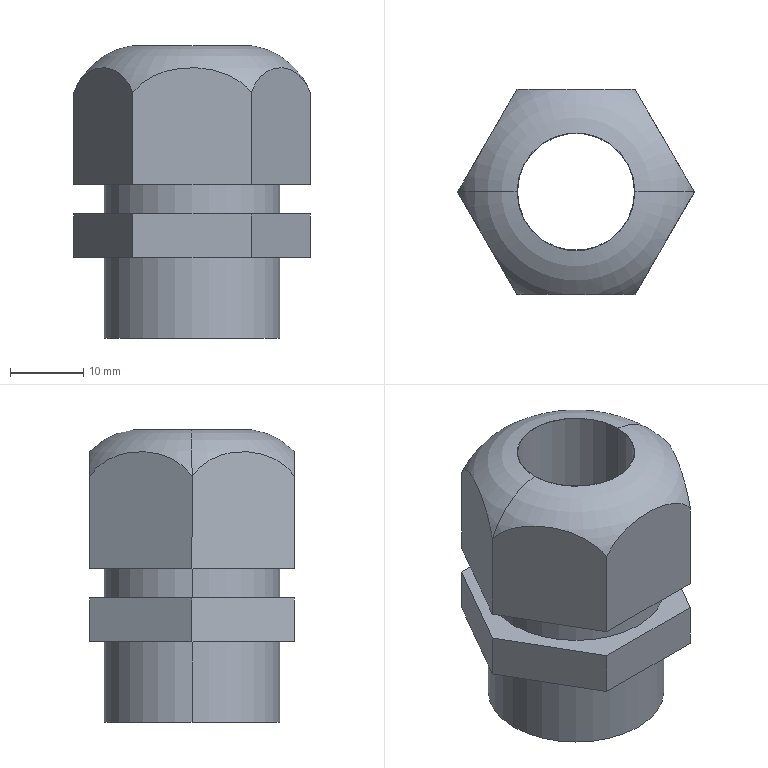Part | SolidWorks | features BaseBody 1 | 1 solid | 29 faces | box 32.332 x 28 x 40 mm | volume 12162 mm3 | plane 17 | cylinder 8 | cone 2 | torus 2 | commonest cylinder face diameters 24 x4 16 x2 20 x2
STEP:
#1=CARTESIAN_POINT('',(10.,0.,24.));
#2=VERTEX_POINT('',#1);
#3=CARTESIAN_POINT('',(-10.,0.,24.));
#4=VERTEX_POINT('',#3);
#5=CARTESIAN_POINT('',(0.,0.,24.));
#6=DIRECTION('',(0.,0.,-1.));
#7=DIRECTION('',(-1.,0.,0.));
#8=AXIS2_PLACEMENT_3D('',#5,#6,#7);
#9=CIRCLE('',#8,10.);
#10=EDGE_CURVE('',#2,#4,#9,.T.);
#11=ORIENTED_EDGE('',*,*,#10,.F.);
#12=CARTESIAN_POINT('',(10.,0.,0.));
#13=VERTEX_POINT('',#12);
#14=CARTESIAN_POINT('',(10.,0.,0.));
#15=DIRECTION('',(0.,0.,-1.));
#16=VECTOR('',#15,1000.);
#17=LINE('',#14,#16);
#18=EDGE_CURVE('',#2,#13,#17,.T.);
#19=ORIENTED_EDGE('',*,*,#18,.T.);
#20=CARTESIAN_POINT('',(-10.,0.,0.));
#21=VERTEX_POINT('',#20);
#22=CARTESIAN_POINT('',(0.,0.,0.));
#23=DIRECTION('',(0.,0.,1.));
#24=DIRECTION('',(-1.,0.,0.));
#25=AXIS2_PLACEMENT_3D('',#22,#23,#24);
#26=CIRCLE('',#25,10.);
#27=EDGE_CURVE('',#21,#13,#26,.T.);
#28=ORIENTED_EDGE('',*,*,#27,.F.);
#29=CARTESIAN_POINT('',(-10.,0.,0.));
#30=DIRECTION('',(0.,0.,-1.));
#31=VECTOR('',#30,1000.);
#32=LINE('',#29,#31);
#33=EDGE_CURVE('',#4,#21,#32,.T.);
#34=ORIENTED_EDGE('',*,*,#33,.F.);
#35=EDGE_LOOP('',(#11,#19,#28,#34));
#36=FACE_OUTER_BOUND('',#35,.T.);
#37=CARTESIAN_POINT('',(0.,0.,0.));
#38=DIRECTION('',(0.,0.,-1.));
#39=DIRECTION('',(-1.,0.,0.));
#40=AXIS2_PLACEMENT_3D('',#37,#38,#39);
#41=CYLINDRICAL_SURFACE('',#40,10.);
#42=ADVANCED_FACE('',(#36),#41,.F.);
#43=CARTESIAN_POINT('',(8.,0.,25.857));
#44=VERTEX_POINT('',#43);
#45=CARTESIAN_POINT('',(-8.,0.,25.857));
#46=VERTEX_POINT('',#45);
#47=CARTESIAN_POINT('',(0.,0.,25.857));
#48=DIRECTION('',(0.,0.,-1.));
#49=DIRECTION('',(1.,0.,0.));
#50=AXIS2_PLACEMENT_3D('',#47,#48,#49);
#51=CIRCLE('',#50,8.);
#52=EDGE_CURVE('',#44,#46,#51,.T.);
#53=ORIENTED_EDGE('',*,*,#52,.F.);
#54=CARTESIAN_POINT('',(10.,0.,24.));
#55=DIRECTION('',(0.7329,0.,-0.6804));
#56=VECTOR('',#55,1000.);
#57=LINE('',#54,#56);
#58=EDGE_CURVE('',#44,#2,#57,.T.);
#59=ORIENTED_EDGE('',*,*,#58,.T.);
#60=ORIENTED_EDGE('',*,*,#10,.T.);
#61=CARTESIAN_POINT('',(-10.,0.,24.));
#62=DIRECTION('',(-0.7329,0.,-0.6804));
#63=VECTOR('',#62,1000.);
#64=LINE('',#61,#63);
#65=EDGE_CURVE('',#46,#4,#64,.T.);
#66=ORIENTED_EDGE('',*,*,#65,.F.);
#67=EDGE_LOOP('',(#53,#59,#60,#66));
#68=FACE_OUTER_BOUND('',#67,.T.);
#69=CARTESIAN_POINT('',(0.,0.,24.));
#70=DIRECTION('',(0.,0.,-1.));
#71=DIRECTION('',(-1.,0.,0.));
#72=AXIS2_PLACEMENT_3D('',#69,#70,#71);
#73=CONICAL_SURFACE('',#72,10.,0.8225);
#74=ADVANCED_FACE('',(#68),#73,.F.);
#75=CARTESIAN_POINT('',(-12.,0.,11.));
#76=VERTEX_POINT('',#75);
#77=CARTESIAN_POINT('',(12.,0.,11.));
#78=VERTEX_POINT('',#77);
#79=CARTESIAN_POINT('',(0.,0.,11.));
#80=DIRECTION('',(0.,0.,-1.));
#81=DIRECTION('',(-1.,0.,0.));
#82=AXIS2_PLACEMENT_3D('',#79,#80,#81);
#83=CIRCLE('',#82,12.);
#84=EDGE_CURVE('',#76,#78,#83,.T.);
#85=ORIENTED_EDGE('',*,*,#84,.T.);
#86=CARTESIAN_POINT('',(12.,0.,0.));
#87=VERTEX_POINT('',#86);
#88=CARTESIAN_POINT('',(12.,0.,0.));
#89=DIRECTION('',(0.,0.,-1.));
#90=VECTOR('',#89,1000.);
#91=LINE('',#88,#90);
#92=EDGE_CURVE('',#78,#87,#91,.T.);
#93=ORIENTED_EDGE('',*,*,#92,.T.);
#94=CARTESIAN_POINT('',(-12.,0.,0.));
#95=VERTEX_POINT('',#94);
#96=CARTESIAN_POINT('',(0.,0.,0.));
#97=DIRECTION('',(0.,0.,1.));
#98=DIRECTION('',(-1.,0.,0.));
#99=AXIS2_PLACEMENT_3D('',#96,#97,#98);
#100=CIRCLE('',#99,12.);
#101=EDGE_CURVE('',#87,#95,#100,.T.);
#102=ORIENTED_EDGE('',*,*,#101,.T.);
#103=CARTESIAN_POINT('',(-12.,0.,0.));
#104=DIRECTION('',(0.,0.,-1.));
#105=VECTOR('',#104,1000.);
#106=LINE('',#103,#105);
#107=EDGE_CURVE('',#76,#95,#106,.T.);
#108=ORIENTED_EDGE('',*,*,#107,.F.);
#109=EDGE_LOOP('',(#85,#93,#102,#108));
#110=FACE_OUTER_BOUND('',#109,.T.);
#111=CARTESIAN_POINT('',(0.,0.,0.));
#112=DIRECTION('',(0.,0.,-1.));
#113=DIRECTION('',(-1.,0.,0.));
#114=AXIS2_PLACEMENT_3D('',#111,#112,#113);
#115=CYLINDRICAL_SURFACE('',#114,12.);
#116=ADVANCED_FACE('',(#110),#115,.T.);
#117=CARTESIAN_POINT('',(8.,0.,40.));
#118=VERTEX_POINT('',#117);
#119=CARTESIAN_POINT('',(-8.,0.,40.));
#120=VERTEX_POINT('',#119);
#121=CARTESIAN_POINT('',(0.,0.,40.));
#122=DIRECTION('',(0.,0.,-1.));
#123=DIRECTION('',(-1.,0.,0.));
#124=AXIS2_PLACEMENT_3D('',#121,#122,#123);
#125=CIRCLE('',#124,8.);
#126=EDGE_CURVE('',#118,#120,#125,.T.);
#127=ORIENTED_EDGE('',*,*,#126,.F.);
#128=CARTESIAN_POINT('',(8.,0.,0.));
#129=DIRECTION('',(0.,0.,-1.));
#130=VECTOR('',#129,1000.);
#131=LINE('',#128,#130);
#132=EDGE_CURVE('',#118,#44,#131,.T.);
#133=ORIENTED_EDGE('',*,*,#132,.T.);
#134=ORIENTED_EDGE('',*,*,#52,.T.);
#135=CARTESIAN_POINT('',(-8.,0.,0.));
#136=DIRECTION('',(0.,0.,-1.));
#137=VECTOR('',#136,1000.);
#138=LINE('',#135,#137);
#139=EDGE_CURVE('',#120,#46,#138,.T.);
#140=ORIENTED_EDGE('',*,*,#139,.F.);
#141=EDGE_LOOP('',(#127,#133,#134,#140));
#142=FACE_OUTER_BOUND('',#141,.T.);
#143=CARTESIAN_POINT('',(0.,0.,0.));
#144=DIRECTION('',(0.,0.,-1.));
#145=DIRECTION('',(-1.,0.,0.));
#146=AXIS2_PLACEMENT_3D('',#143,#144,#145);
#147=CYLINDRICAL_SURFACE('',#146,8.);
#148=ADVANCED_FACE('',(#142),#147,.F.);
#149=CARTESIAN_POINT('',(-8.083,14.,33.63));
#150=VERTEX_POINT('',#149);
#151=CARTESIAN_POINT('',(-16.166,0.,33.63));
#152=VERTEX_POINT('',#151);
#153=CARTESIAN_POINT('',(-8.083,14.,33.63));
#154=CARTESIAN_POINT('',(-8.319,13.591,34.231));
#155=CARTESIAN_POINT('',(-8.596,13.111,34.735));
#156=CARTESIAN_POINT('',(-9.061,12.306,35.379));
#157=CARTESIAN_POINT('',(-9.225,12.022,35.575));
#158=CARTESIAN_POINT('',(-9.561,11.44,35.924));
#159=CARTESIAN_POINT('',(-9.733,11.142,36.078));
#160=CARTESIAN_POINT('',(-10.085,10.532,36.347));
#161=CARTESIAN_POINT('',(-10.265,10.221,36.463));
#162=CARTESIAN_POINT('',(-10.631,9.586,36.661));
#163=CARTESIAN_POINT('',(-10.817,9.265,36.742));
#164=CARTESIAN_POINT('',(-11.373,8.301,36.933));
#165=CARTESIAN_POINT('',(-11.746,7.655,36.994));
#166=CARTESIAN_POINT('',(-12.498,6.353,36.995));
#167=CARTESIAN_POINT('',(-12.879,5.693,36.932));
#168=CARTESIAN_POINT('',(-13.619,4.411,36.677));
#169=CARTESIAN_POINT('',(-13.98,3.786,36.486));
#170=CARTESIAN_POINT('',(-14.506,2.875,36.086));
#171=CARTESIAN_POINT('',(-14.679,2.576,35.933));
#172=CARTESIAN_POINT('',(-15.017,1.989,35.583));
#173=CARTESIAN_POINT('',(-15.18,1.707,35.389));
#174=CARTESIAN_POINT('',(-15.49,1.17,34.961));
#175=CARTESIAN_POINT('',(-15.638,0.914,34.726));
#176=CARTESIAN_POINT('',(-15.917,0.4313,34.212));
#177=CARTESIAN_POINT('',(-16.048,0.2045,33.931));
#178=CARTESIAN_POINT('',(-16.166,0.,33.63));
#179=B_SPLINE_CURVE_WITH_KNOTS('',3,(#153,#154,#155,#156,#157,#158,#159,#160,#161,#162,#163,#164,#165,#166,#167,#168,#169,#170,#171,#172,#173,#174,#175,#176,#177,#178),.UNSPECIFIED.,.F.,.F.,(4,2,2,2,2,2,2,2,2,2,2,2,4),(0.,0.002248,0.003373,0.004497,0.005621,0.006745,0.008994,0.01124,0.01349,0.01461,0.01574,0.01686,0.01799),.UNSPECIFIED.);
#180=EDGE_CURVE('',#150,#152,#179,.T.);
#181=ORIENTED_EDGE('',*,*,#180,.T.);
#182=CARTESIAN_POINT('',(-8.052,0.,40.));
#183=VERTEX_POINT('',#182);
#184=CARTESIAN_POINT('',(-6.686,0.,29.907));
#185=DIRECTION('',(0.,1.,0.));
#186=DIRECTION('',(-1.,0.,0.));
#187=AXIS2_PLACEMENT_3D('',#184,#185,#186);
#188=CIRCLE('',#187,10.185);
#189=EDGE_CURVE('',#152,#183,#188,.T.);
#190=ORIENTED_EDGE('',*,*,#189,.T.);
#191=CARTESIAN_POINT('',(8.052,0.,40.));
#192=VERTEX_POINT('',#191);
#193=CARTESIAN_POINT('',(0.,0.,40.));
#194=DIRECTION('',(0.,0.,1.));
#195=DIRECTION('',(1.,0.,0.));
#196=AXIS2_PLACEMENT_3D('',#193,#194,#195);
#197=CIRCLE('',#196,8.052);
#198=EDGE_CURVE('',#192,#183,#197,.T.);
#199=ORIENTED_EDGE('',*,*,#198,.F.);
#200=CARTESIAN_POINT('',(16.166,0.,33.63));
#201=VERTEX_POINT('',#200);
#202=CARTESIAN_POINT('',(6.686,0.,29.907));
#203=DIRECTION('',(0.,-1.,0.));
#204=DIRECTION('',(0.,0.,-1.));
#205=AXIS2_PLACEMENT_3D('',#202,#203,#204);
#206=CIRCLE('',#205,10.185);
#207=EDGE_CURVE('',#201,#192,#206,.T.);
#208=ORIENTED_EDGE('',*,*,#207,.F.);
#209=CARTESIAN_POINT('',(8.083,14.,33.63));
#210=VERTEX_POINT('',#209);
#211=CARTESIAN_POINT('',(16.166,0.,33.63));
#212=CARTESIAN_POINT('',(15.93,0.4089,34.231));
#213=CARTESIAN_POINT('',(15.652,0.8894,34.735));
#214=CARTESIAN_POINT('',(15.188,1.694,35.379));
#215=CARTESIAN_POINT('',(15.024,1.978,35.575));
#216=CARTESIAN_POINT('',(14.688,2.56,35.924));
#217=CARTESIAN_POINT('',(14.516,2.858,36.078));
#218=CARTESIAN_POINT('',(14.164,3.468,36.347));
#219=CARTESIAN_POINT('',(13.984,3.779,36.463));
#220=CARTESIAN_POINT('',(13.618,4.414,36.661));
#221=CARTESIAN_POINT('',(13.432,4.735,36.742));
#222=CARTESIAN_POINT('',(12.876,5.699,36.933));
#223=CARTESIAN_POINT('',(12.502,6.345,36.994));
#224=CARTESIAN_POINT('',(11.751,7.647,36.995));
#225=CARTESIAN_POINT('',(11.37,8.307,36.932));
#226=CARTESIAN_POINT('',(10.63,9.589,36.677));
#227=CARTESIAN_POINT('',(10.269,10.214,36.486));
#228=CARTESIAN_POINT('',(9.743,11.125,36.086));
#229=CARTESIAN_POINT('',(9.57,11.424,35.933));
#230=CARTESIAN_POINT('',(9.231,12.011,35.583));
#231=CARTESIAN_POINT('',(9.069,12.293,35.389));
#232=CARTESIAN_POINT('',(8.758,12.83,34.961));
#233=CARTESIAN_POINT('',(8.611,13.086,34.726));
#234=CARTESIAN_POINT('',(8.332,13.569,34.212));
#235=CARTESIAN_POINT('',(8.201,13.795,33.931));
#236=CARTESIAN_POINT('',(8.083,14.,33.63));
#237=B_SPLINE_CURVE_WITH_KNOTS('',3,(#211,#212,#213,#214,#215,#216,#217,#218,#219,#220,#221,#222,#223,#224,#225,#226,#227,#228,#229,#230,#231,#232,#233,#234,#235,#236),.UNSPECIFIED.,.F.,.F.,(4,2,2,2,2,2,2,2,2,2,2,2,4),(0.,0.002248,0.003373,0.004497,0.005621,0.006745,0.008994,0.01124,0.01349,0.01461,0.01574,0.01686,0.01799),.UNSPECIFIED.);
#238=EDGE_CURVE('',#201,#210,#237,.T.);
#239=ORIENTED_EDGE('',*,*,#238,.T.);
#240=CARTESIAN_POINT('',(8.083,14.,33.63));
#241=CARTESIAN_POINT('',(7.611,14.,34.231));
#242=CARTESIAN_POINT('',(7.056,14.,34.735));
#243=CARTESIAN_POINT('',(6.127,14.,35.379));
#244=CARTESIAN_POINT('',(5.799,14.,35.575));
#245=CARTESIAN_POINT('',(5.127,14.,35.924));
#246=CARTESIAN_POINT('',(4.782,14.,36.078));
#247=CARTESIAN_POINT('',(4.078,14.,36.347));
#248=CARTESIAN_POINT('',(3.719,14.,36.463));
#249=CARTESIAN_POINT('',(2.986,14.,36.661));
#250=CARTESIAN_POINT('',(2.615,14.,36.742));
#251=CARTESIAN_POINT('',(1.503,14.,36.933));
#252=CARTESIAN_POINT('',(0.7559,14.,36.994));
#253=CARTESIAN_POINT('',(-0.7471,14.,36.995));
#254=CARTESIAN_POINT('',(-1.51,14.,36.932));
#255=CARTESIAN_POINT('',(-2.989,14.,36.677));
#256=CARTESIAN_POINT('',(-3.711,14.,36.486));
#257=CARTESIAN_POINT('',(-4.763,14.,36.086));
#258=CARTESIAN_POINT('',(-5.109,14.,35.933));
#259=CARTESIAN_POINT('',(-5.786,14.,35.583));
#260=CARTESIAN_POINT('',(-6.111,14.,35.389));
#261=CARTESIAN_POINT('',(-6.732,14.,34.961));
#262=CARTESIAN_POINT('',(-7.027,14.,34.726));
#263=CARTESIAN_POINT('',(-7.585,14.,34.212));
#264=CARTESIAN_POINT('',(-7.847,14.,33.931));
#265=CARTESIAN_POINT('',(-8.083,14.,33.63));
#266=B_SPLINE_CURVE_WITH_KNOTS('',3,(#240,#241,#242,#243,#244,#245,#246,#247,#248,#249,#250,#251,#252,#253,#254,#255,#256,#257,#258,#259,#260,#261,#262,#263,#264,#265),.UNSPECIFIED.,.F.,.F.,(4,2,2,2,2,2,2,2,2,2,2,2,4),(0.,0.002248,0.003373,0.004497,0.005621,0.006745,0.008994,0.01124,0.01349,0.01461,0.01574,0.01686,0.01799),.UNSPECIFIED.);
#267=EDGE_CURVE('',#210,#150,#266,.T.);
#268=ORIENTED_EDGE('',*,*,#267,.T.);
#269=EDGE_LOOP('',(#181,#190,#199,#208,#239,#268));
#270=FACE_OUTER_BOUND('',#269,.T.);
#271=CARTESIAN_POINT('',(0.,0.,29.907));
#272=DIRECTION('',(0.,0.,1.));
#273=DIRECTION('',(1.,0.,0.));
#274=AXIS2_PLACEMENT_3D('',#271,#272,#273);
#275=TOROIDAL_SURFACE('',#274,6.686,10.185);
#276=ADVANCED_FACE('',(#270),#275,.T.);
#277=CARTESIAN_POINT('',(-12.,0.,21.));
#278=VERTEX_POINT('',#277);
#279=CARTESIAN_POINT('',(12.,0.,21.));
#280=VERTEX_POINT('',#279);
#281=CARTESIAN_POINT('',(0.,0.,21.));
#282=DIRECTION('',(0.,0.,-1.));
#283=DIRECTION('',(-1.,0.,0.));
#284=AXIS2_PLACEMENT_3D('',#281,#282,#283);
#285=CIRCLE('',#284,12.);
#286=EDGE_CURVE('',#278,#280,#285,.T.);
#287=ORIENTED_EDGE('',*,*,#286,.T.);
#288=CARTESIAN_POINT('',(12.,0.,17.));
#289=VERTEX_POINT('',#288);
#290=CARTESIAN_POINT('',(12.,0.,0.));
#291=DIRECTION('',(0.,0.,-1.));
#292=VECTOR('',#291,1000.);
#293=LINE('',#290,#292);
#294=EDGE_CURVE('',#280,#289,#293,.T.);
#295=ORIENTED_EDGE('',*,*,#294,.T.);
#296=CARTESIAN_POINT('',(-12.,0.,17.));
#297=VERTEX_POINT('',#296);
#298=CARTESIAN_POINT('',(0.,0.,17.));
#299=DIRECTION('',(0.,0.,1.));
#300=DIRECTION('',(-1.,0.,0.));
#301=AXIS2_PLACEMENT_3D('',#298,#299,#300);
#302=CIRCLE('',#301,12.);
#303=EDGE_CURVE('',#289,#297,#302,.T.);
#304=ORIENTED_EDGE('',*,*,#303,.T.);
#305=CARTESIAN_POINT('',(-12.,0.,0.));
#306=DIRECTION('',(0.,0.,-1.));
#307=VECTOR('',#306,1000.);
#308=LINE('',#305,#307);
#309=EDGE_CURVE('',#278,#297,#308,.T.);
#310=ORIENTED_EDGE('',*,*,#309,.F.);
#311=EDGE_LOOP('',(#287,#295,#304,#310));
#312=FACE_OUTER_BOUND('',#311,.T.);
#313=CARTESIAN_POINT('',(0.,0.,0.));
#314=DIRECTION('',(0.,0.,-1.));
#315=DIRECTION('',(-1.,0.,0.));
#316=AXIS2_PLACEMENT_3D('',#313,#314,#315);
#317=CYLINDRICAL_SURFACE('',#316,12.);
#318=ADVANCED_FACE('',(#312),#317,.T.);
#319=ORIENTED_EDGE('',*,*,#18,.F.);
#320=CARTESIAN_POINT('',(0.,0.,24.));
#321=DIRECTION('',(0.,0.,-1.));
#322=DIRECTION('',(-1.,0.,0.));
#323=AXIS2_PLACEMENT_3D('',#320,#321,#322);
#324=CIRCLE('',#323,10.);
#325=EDGE_CURVE('',#4,#2,#324,.T.);
#326=ORIENTED_EDGE('',*,*,#325,.F.);
#327=ORIENTED_EDGE('',*,*,#33,.T.);
#328=CARTESIAN_POINT('',(0.,0.,0.));
#329=DIRECTION('',(0.,0.,1.));
#330=DIRECTION('',(-1.,0.,0.));
#331=AXIS2_PLACEMENT_3D('',#328,#329,#330);
#332=CIRCLE('',#331,10.);
#333=EDGE_CURVE('',#13,#21,#332,.T.);
#334=ORIENTED_EDGE('',*,*,#333,.F.);
#335=EDGE_LOOP('',(#319,#326,#327,#334));
#336=FACE_OUTER_BOUND('',#335,.T.);
#337=CARTESIAN_POINT('',(0.,0.,0.));
#338=DIRECTION('',(0.,0.,-1.));
#339=DIRECTION('',(-1.,0.,0.));
#340=AXIS2_PLACEMENT_3D('',#337,#338,#339);
#341=CYLINDRICAL_SURFACE('',#340,10.);
#342=ADVANCED_FACE('',(#336),#341,.F.);
#343=ORIENTED_EDGE('',*,*,#27,.T.);
#344=ORIENTED_EDGE('',*,*,#333,.T.);
#345=EDGE_LOOP('',(#343,#344));
#346=FACE_BOUND('',#345,.T.);
#347=CARTESIAN_POINT('',(0.,0.,0.));
#348=DIRECTION('',(0.,0.,1.));
#349=DIRECTION('',(-1.,0.,0.));
#350=AXIS2_PLACEMENT_3D('',#347,#348,#349);
#351=CIRCLE('',#350,12.);
#352=EDGE_CURVE('',#95,#87,#351,.T.);
#353=ORIENTED_EDGE('',*,*,#352,.F.);
#354=ORIENTED_EDGE('',*,*,#101,.F.);
#355=EDGE_LOOP('',(#353,#354));
#356=FACE_OUTER_BOUND('',#355,.T.);
#357=CARTESIAN_POINT('',(-16.166,-14.,0.));
#358=DIRECTION('',(0.,0.,1.));
#359=DIRECTION('',(1.,0.,0.));
#360=AXIS2_PLACEMENT_3D('',#357,#358,#359);
#361=PLANE('',#360);
#362=ADVANCED_FACE('',(#346,#356),#361,.F.);
#363=ORIENTED_EDGE('',*,*,#58,.F.);
#364=CARTESIAN_POINT('',(0.,0.,25.857));
#365=DIRECTION('',(0.,0.,-1.));
#366=DIRECTION('',(1.,0.,0.));
#367=AXIS2_PLACEMENT_3D('',#364,#365,#366);
#368=CIRCLE('',#367,8.);
#369=EDGE_CURVE('',#46,#44,#368,.T.);
#370=ORIENTED_EDGE('',*,*,#369,.F.);
#371=ORIENTED_EDGE('',*,*,#65,.T.);
#372=ORIENTED_EDGE('',*,*,#325,.T.);
#373=EDGE_LOOP('',(#363,#370,#371,#372));
#374=FACE_OUTER_BOUND('',#373,.T.);
#375=CARTESIAN_POINT('',(0.,0.,24.));
#376=DIRECTION('',(0.,0.,-1.));
#377=DIRECTION('',(-1.,0.,0.));
#378=AXIS2_PLACEMENT_3D('',#375,#376,#377);
#379=CONICAL_SURFACE('',#378,10.,0.8225);
#380=ADVANCED_FACE('',(#374),#379,.F.);
#381=ORIENTED_EDGE('',*,*,#92,.F.);
#382=CARTESIAN_POINT('',(0.,0.,11.));
#383=DIRECTION('',(0.,0.,-1.));
#384=DIRECTION('',(-1.,0.,0.));
#385=AXIS2_PLACEMENT_3D('',#382,#383,#384);
#386=CIRCLE('',#385,12.);
#387=EDGE_CURVE('',#78,#76,#386,.T.);
#388=ORIENTED_EDGE('',*,*,#387,.T.);
#389=ORIENTED_EDGE('',*,*,#107,.T.);
#390=ORIENTED_EDGE('',*,*,#352,.T.);
#391=EDGE_LOOP('',(#381,#388,#389,#390));
#392=FACE_OUTER_BOUND('',#391,.T.);
#393=CARTESIAN_POINT('',(0.,0.,0.));
#394=DIRECTION('',(0.,0.,-1.));
#395=DIRECTION('',(-1.,0.,0.));
#396=AXIS2_PLACEMENT_3D('',#393,#394,#395);
#397=CYLINDRICAL_SURFACE('',#396,12.);
#398=ADVANCED_FACE('',(#392),#397,.T.);
#399=ORIENTED_EDGE('',*,*,#132,.F.);
#400=CARTESIAN_POINT('',(0.,0.,40.));
#401=DIRECTION('',(0.,0.,-1.));
#402=DIRECTION('',(-1.,0.,0.));
#403=AXIS2_PLACEMENT_3D('',#400,#401,#402);
#404=CIRCLE('',#403,8.);
#405=EDGE_CURVE('',#120,#118,#404,.T.);
#406=ORIENTED_EDGE('',*,*,#405,.F.);
#407=ORIENTED_EDGE('',*,*,#139,.T.);
#408=ORIENTED_EDGE('',*,*,#369,.T.);
#409=EDGE_LOOP('',(#399,#406,#407,#408));
#410=FACE_OUTER_BOUND('',#409,.T.);
#411=CARTESIAN_POINT('',(0.,0.,0.));
#412=DIRECTION('',(0.,0.,-1.));
#413=DIRECTION('',(-1.,0.,0.));
#414=AXIS2_PLACEMENT_3D('',#411,#412,#413);
#415=CYLINDRICAL_SURFACE('',#414,8.);
#416=ADVANCED_FACE('',(#410),#415,.F.);
#417=CARTESIAN_POINT('',(-16.166,0.,11.));
#418=VERTEX_POINT('',#417);
#419=CARTESIAN_POINT('',(-8.083,-14.,11.));
#420=VERTEX_POINT('',#419);
#421=CARTESIAN_POINT('',(-16.166,0.,11.));
#422=DIRECTION('',(0.5,-0.866,0.));
#423=VECTOR('',#422,1000.);
#424=LINE('',#421,#423);
#425=EDGE_CURVE('',#418,#420,#424,.T.);
#426=ORIENTED_EDGE('',*,*,#425,.F.);
#427=CARTESIAN_POINT('',(-8.083,14.,11.));
#428=VERTEX_POINT('',#427);
#429=CARTESIAN_POINT('',(-8.083,14.,11.));
#430=DIRECTION('',(-0.5,-0.866,0.));
#431=VECTOR('',#430,1000.);
#432=LINE('',#429,#431);
#433=EDGE_CURVE('',#428,#418,#432,.T.);
#434=ORIENTED_EDGE('',*,*,#433,.F.);
#435=CARTESIAN_POINT('',(8.083,14.,11.));
#436=VERTEX_POINT('',#435);
#437=CARTESIAN_POINT('',(0.,14.,11.));
#438=DIRECTION('',(-1.,0.,0.));
#439=VECTOR('',#438,1000.);
#440=LINE('',#437,#439);
#441=EDGE_CURVE('',#436,#428,#440,.T.);
#442=ORIENTED_EDGE('',*,*,#441,.F.);
#443=CARTESIAN_POINT('',(16.166,0.,11.));
#444=VERTEX_POINT('',#443);
#445=CARTESIAN_POINT('',(16.166,0.,11.));
#446=DIRECTION('',(-0.5,0.866,0.));
#447=VECTOR('',#446,1000.);
#448=LINE('',#445,#447);
#449=EDGE_CURVE('',#444,#436,#448,.T.);
#450=ORIENTED_EDGE('',*,*,#449,.F.);
#451=CARTESIAN_POINT('',(8.083,-14.,11.));
#452=VERTEX_POINT('',#451);
#453=CARTESIAN_POINT('',(8.083,-14.,11.));
#454=DIRECTION('',(0.5,0.866,0.));
#455=VECTOR('',#454,1000.);
#456=LINE('',#453,#455);
#457=EDGE_CURVE('',#452,#444,#456,.T.);
#458=ORIENTED_EDGE('',*,*,#457,.F.);
#459=CARTESIAN_POINT('',(0.,-14.,11.));
#460=DIRECTION('',(1.,0.,0.));
#461=VECTOR('',#460,1000.);
#462=LINE('',#459,#461);
#463=EDGE_CURVE('',#420,#452,#462,.T.);
#464=ORIENTED_EDGE('',*,*,#463,.F.);
#465=EDGE_LOOP('',(#426,#434,#442,#450,#458,#464));
#466=FACE_OUTER_BOUND('',#465,.T.);
#467=ORIENTED_EDGE('',*,*,#84,.F.);
#468=ORIENTED_EDGE('',*,*,#387,.F.);
#469=EDGE_LOOP('',(#467,#468));
#470=FACE_BOUND('',#469,.T.);
#471=CARTESIAN_POINT('',(0.,-19.143,11.));
#472=DIRECTION('',(0.,0.,1.));
#473=DIRECTION('',(1.,0.,0.));
#474=AXIS2_PLACEMENT_3D('',#471,#472,#473);
#475=PLANE('',#474);
#476=ADVANCED_FACE('',(#466,#470),#475,.F.);
#477=ORIENTED_EDGE('',*,*,#198,.T.);
#478=CARTESIAN_POINT('',(0.,0.,40.));
#479=DIRECTION('',(0.,0.,1.));
#480=DIRECTION('',(1.,0.,0.));
#481=AXIS2_PLACEMENT_3D('',#478,#479,#480);
#482=CIRCLE('',#481,8.052);
#483=EDGE_CURVE('',#183,#192,#482,.T.);
#484=ORIENTED_EDGE('',*,*,#483,.T.);
#485=EDGE_LOOP('',(#477,#484));
#486=FACE_OUTER_BOUND('',#485,.T.);
#487=ORIENTED_EDGE('',*,*,#405,.T.);
#488=ORIENTED_EDGE('',*,*,#126,.T.);
#489=EDGE_LOOP('',(#487,#488));
#490=FACE_BOUND('',#489,.T.);
#491=CARTESIAN_POINT('',(-16.166,-14.,40.));
#492=DIRECTION('',(0.,0.,1.));
#493=DIRECTION('',(1.,0.,0.));
#494=AXIS2_PLACEMENT_3D('',#491,#492,#493);
#495=PLANE('',#494);
#496=ADVANCED_FACE('',(#486,#490),#495,.T.);
#497=ORIENTED_EDGE('',*,*,#463,.T.);
#498=CARTESIAN_POINT('',(8.083,-14.,17.));
#499=VERTEX_POINT('',#498);
#500=CARTESIAN_POINT('',(8.083,-14.,40.));
#501=DIRECTION('',(0.,0.,-1.));
#502=VECTOR('',#501,1000.);
#503=LINE('',#500,#502);
#504=EDGE_CURVE('',#499,#452,#503,.T.);
#505=ORIENTED_EDGE('',*,*,#504,.F.);
#506=CARTESIAN_POINT('',(-8.083,-14.,17.));
#507=VERTEX_POINT('',#506);
#508=CARTESIAN_POINT('',(-8.083,-14.,17.));
#509=DIRECTION('',(1.,0.,0.));
#510=VECTOR('',#509,1000.);
#511=LINE('',#508,#510);
#512=EDGE_CURVE('',#507,#499,#511,.T.);
#513=ORIENTED_EDGE('',*,*,#512,.F.);
#514=CARTESIAN_POINT('',(-8.083,-14.,40.));
#515=DIRECTION('',(0.,0.,1.));
#516=VECTOR('',#515,1000.);
#517=LINE('',#514,#516);
#518=EDGE_CURVE('',#420,#507,#517,.T.);
#519=ORIENTED_EDGE('',*,*,#518,.F.);
#520=EDGE_LOOP('',(#497,#505,#513,#519));
#521=FACE_OUTER_BOUND('',#520,.T.);
#522=CARTESIAN_POINT('',(-8.083,-14.,40.));
#523=DIRECTION('',(0.,1.,0.));
#524=DIRECTION('',(-1.,0.,0.));
#525=AXIS2_PLACEMENT_3D('',#522,#523,#524);
#526=PLANE('',#525);
#527=ADVANCED_FACE('',(#521),#526,.F.);
#528=ORIENTED_EDGE('',*,*,#425,.T.);
#529=ORIENTED_EDGE('',*,*,#518,.T.);
#530=CARTESIAN_POINT('',(-16.166,0.,17.));
#531=VERTEX_POINT('',#530);
#532=CARTESIAN_POINT('',(-16.166,0.,17.));
#533=DIRECTION('',(0.5,-0.866,0.));
#534=VECTOR('',#533,1000.);
#535=LINE('',#532,#534);
#536=EDGE_CURVE('',#531,#507,#535,.T.);
#537=ORIENTED_EDGE('',*,*,#536,.F.);
#538=CARTESIAN_POINT('',(-16.166,0.,40.));
#539=DIRECTION('',(0.,0.,1.));
#540=VECTOR('',#539,1000.);
#541=LINE('',#538,#540);
#542=EDGE_CURVE('',#418,#531,#541,.T.);
#543=ORIENTED_EDGE('',*,*,#542,.F.);
#544=EDGE_LOOP('',(#528,#529,#537,#543));
#545=FACE_OUTER_BOUND('',#544,.T.);
#546=CARTESIAN_POINT('',(-16.166,0.,40.));
#547=DIRECTION('',(0.866,0.5,0.));
#548=DIRECTION('',(-0.5,0.866,0.));
#549=AXIS2_PLACEMENT_3D('',#546,#547,#548);
#550=PLANE('',#549);
#551=ADVANCED_FACE('',(#545),#550,.F.);
#552=ORIENTED_EDGE('',*,*,#433,.T.);
#553=ORIENTED_EDGE('',*,*,#542,.T.);
#554=CARTESIAN_POINT('',(-8.083,14.,17.));
#555=VERTEX_POINT('',#554);
#556=CARTESIAN_POINT('',(-8.083,14.,17.));
#557=DIRECTION('',(-0.5,-0.866,0.));
#558=VECTOR('',#557,1000.);
#559=LINE('',#556,#558);
#560=EDGE_CURVE('',#555,#531,#559,.T.);
#561=ORIENTED_EDGE('',*,*,#560,.F.);
#562=CARTESIAN_POINT('',(-8.083,14.,40.));
#563=DIRECTION('',(0.,0.,1.));
#564=VECTOR('',#563,1000.);
#565=LINE('',#562,#564);
#566=EDGE_CURVE('',#428,#555,#565,.T.);
#567=ORIENTED_EDGE('',*,*,#566,.F.);
#568=EDGE_LOOP('',(#552,#553,#561,#567));
#569=FACE_OUTER_BOUND('',#568,.T.);
#570=CARTESIAN_POINT('',(-8.083,14.,40.));
#571=DIRECTION('',(0.866,-0.5,0.));
#572=DIRECTION('',(0.5,0.866,0.));
#573=AXIS2_PLACEMENT_3D('',#570,#571,#572);
#574=PLANE('',#573);
#575=ADVANCED_FACE('',(#569),#574,.F.);
#576=ORIENTED_EDGE('',*,*,#441,.T.);
#577=ORIENTED_EDGE('',*,*,#566,.T.);
#578=CARTESIAN_POINT('',(8.083,14.,17.));
#579=VERTEX_POINT('',#578);
#580=CARTESIAN_POINT('',(8.083,14.,17.));
#581=DIRECTION('',(-1.,0.,0.));
#582=VECTOR('',#581,1000.);
#583=LINE('',#580,#582);
#584=EDGE_CURVE('',#579,#555,#583,.T.);
#585=ORIENTED_EDGE('',*,*,#584,.F.);
#586=CARTESIAN_POINT('',(8.083,14.,40.));
#587=DIRECTION('',(0.,0.,1.));
#588=VECTOR('',#587,1000.);
#589=LINE('',#586,#588);
#590=EDGE_CURVE('',#436,#579,#589,.T.);
#591=ORIENTED_EDGE('',*,*,#590,.F.);
#592=EDGE_LOOP('',(#576,#577,#585,#591));
#593=FACE_OUTER_BOUND('',#592,.T.);
#594=CARTESIAN_POINT('',(8.083,14.,40.));
#595=DIRECTION('',(0.,-1.,0.));
#596=DIRECTION('',(1.,0.,0.));
#597=AXIS2_PLACEMENT_3D('',#594,#595,#596);
#598=PLANE('',#597);
#599=ADVANCED_FACE('',(#593),#598,.F.);
#600=ORIENTED_EDGE('',*,*,#449,.T.);
#601=ORIENTED_EDGE('',*,*,#590,.T.);
#602=CARTESIAN_POINT('',(16.166,0.,17.));
#603=VERTEX_POINT('',#602);
#604=CARTESIAN_POINT('',(16.166,0.,17.));
#605=DIRECTION('',(-0.5,0.866,0.));
#606=VECTOR('',#605,1000.);
#607=LINE('',#604,#606);
#608=EDGE_CURVE('',#603,#579,#607,.T.);
#609=ORIENTED_EDGE('',*,*,#608,.F.);
#610=CARTESIAN_POINT('',(16.166,0.,40.));
#611=DIRECTION('',(0.,0.,1.));
#612=VECTOR('',#611,1000.);
#613=LINE('',#610,#612);
#614=EDGE_CURVE('',#444,#603,#613,.T.);
#615=ORIENTED_EDGE('',*,*,#614,.F.);
#616=EDGE_LOOP('',(#600,#601,#609,#615));
#617=FACE_OUTER_BOUND('',#616,.T.);
#618=CARTESIAN_POINT('',(16.166,0.,40.));
#619=DIRECTION('',(-0.866,-0.5,0.));
#620=DIRECTION('',(0.5,-0.866,0.));
#621=AXIS2_PLACEMENT_3D('',#618,#619,#620);
#622=PLANE('',#621);
#623=ADVANCED_FACE('',(#617),#622,.F.);
#624=ORIENTED_EDGE('',*,*,#457,.T.);
#625=ORIENTED_EDGE('',*,*,#614,.T.);
#626=CARTESIAN_POINT('',(8.083,-14.,17.));
#627=DIRECTION('',(0.5,0.866,0.));
#628=VECTOR('',#627,1000.);
#629=LINE('',#626,#628);
#630=EDGE_CURVE('',#499,#603,#629,.T.);
#631=ORIENTED_EDGE('',*,*,#630,.F.);
#632=ORIENTED_EDGE('',*,*,#504,.T.);
#633=EDGE_LOOP('',(#624,#625,#631,#632));
#634=FACE_OUTER_BOUND('',#633,.T.);
#635=CARTESIAN_POINT('',(8.083,-14.,40.));
#636=DIRECTION('',(-0.866,0.5,0.));
#637=DIRECTION('',(-0.5,-0.866,0.));
#638=AXIS2_PLACEMENT_3D('',#635,#636,#637);
#639=PLANE('',#638);
#640=ADVANCED_FACE('',(#634),#639,.F.);
#641=ORIENTED_EDGE('',*,*,#189,.F.);
#642=CARTESIAN_POINT('',(-8.083,-14.,33.63));
#643=VERTEX_POINT('',#642);
#644=CARTESIAN_POINT('',(-16.166,0.,33.63));
#645=CARTESIAN_POINT('',(-15.93,-0.4089,34.231));
#646=CARTESIAN_POINT('',(-15.652,-0.8894,34.735));
#647=CARTESIAN_POINT('',(-15.188,-1.694,35.379));
#648=CARTESIAN_POINT('',(-15.024,-1.978,35.575));
#649=CARTESIAN_POINT('',(-14.688,-2.56,35.924));
#650=CARTESIAN_POINT('',(-14.516,-2.858,36.078));
#651=CARTESIAN_POINT('',(-14.164,-3.468,36.347));
#652=CARTESIAN_POINT('',(-13.984,-3.779,36.463));
#653=CARTESIAN_POINT('',(-13.618,-4.414,36.661));
#654=CARTESIAN_POINT('',(-13.432,-4.735,36.742));
#655=CARTESIAN_POINT('',(-12.876,-5.699,36.933));
#656=CARTESIAN_POINT('',(-12.502,-6.345,36.994));
#657=CARTESIAN_POINT('',(-11.751,-7.647,36.995));
#658=CARTESIAN_POINT('',(-11.37,-8.307,36.932));
#659=CARTESIAN_POINT('',(-10.63,-9.589,36.677));
#660=CARTESIAN_POINT('',(-10.269,-10.214,36.486));
#661=CARTESIAN_POINT('',(-9.743,-11.125,36.086));
#662=CARTESIAN_POINT('',(-9.57,-11.424,35.933));
#663=CARTESIAN_POINT('',(-9.231,-12.011,35.583));
#664=CARTESIAN_POINT('',(-9.069,-12.293,35.389));
#665=CARTESIAN_POINT('',(-8.758,-12.83,34.961));
#666=CARTESIAN_POINT('',(-8.611,-13.086,34.726));
#667=CARTESIAN_POINT('',(-8.332,-13.569,34.212));
#668=CARTESIAN_POINT('',(-8.201,-13.795,33.931));
#669=CARTESIAN_POINT('',(-8.083,-14.,33.63));
#670=B_SPLINE_CURVE_WITH_KNOTS('',3,(#644,#645,#646,#647,#648,#649,#650,#651,#652,#653,#654,#655,#656,#657,#658,#659,#660,#661,#662,#663,#664,#665,#666,#667,#668,#669),.UNSPECIFIED.,.F.,.F.,(4,2,2,2,2,2,2,2,2,2,2,2,4),(0.,0.002248,0.003373,0.004497,0.005621,0.006745,0.008994,0.01124,0.01349,0.01461,0.01574,0.01686,0.01799),.UNSPECIFIED.);
#671=EDGE_CURVE('',#152,#643,#670,.T.);
#672=ORIENTED_EDGE('',*,*,#671,.T.);
#673=CARTESIAN_POINT('',(8.083,-14.,33.63));
#674=VERTEX_POINT('',#673);
#675=CARTESIAN_POINT('',(-8.083,-14.,33.63));
#676=CARTESIAN_POINT('',(-7.611,-14.,34.231));
#677=CARTESIAN_POINT('',(-7.056,-14.,34.735));
#678=CARTESIAN_POINT('',(-6.127,-14.,35.379));
#679=CARTESIAN_POINT('',(-5.799,-14.,35.575));
#680=CARTESIAN_POINT('',(-5.127,-14.,35.924));
#681=CARTESIAN_POINT('',(-4.782,-14.,36.078));
#682=CARTESIAN_POINT('',(-4.078,-14.,36.347));
#683=CARTESIAN_POINT('',(-3.719,-14.,36.463));
#684=CARTESIAN_POINT('',(-2.986,-14.,36.661));
#685=CARTESIAN_POINT('',(-2.615,-14.,36.742));
#686=CARTESIAN_POINT('',(-1.503,-14.,36.933));
#687=CARTESIAN_POINT('',(-0.7559,-14.,36.994));
#688=CARTESIAN_POINT('',(0.7471,-14.,36.995));
#689=CARTESIAN_POINT('',(1.51,-14.,36.932));
#690=CARTESIAN_POINT('',(2.989,-14.,36.677));
#691=CARTESIAN_POINT('',(3.711,-14.,36.486));
#692=CARTESIAN_POINT('',(4.763,-14.,36.086));
#693=CARTESIAN_POINT('',(5.109,-14.,35.933));
#694=CARTESIAN_POINT('',(5.786,-14.,35.583));
#695=CARTESIAN_POINT('',(6.111,-14.,35.389));
#696=CARTESIAN_POINT('',(6.732,-14.,34.961));
#697=CARTESIAN_POINT('',(7.027,-14.,34.726));
#698=CARTESIAN_POINT('',(7.585,-14.,34.212));
#699=CARTESIAN_POINT('',(7.847,-14.,33.931));
#700=CARTESIAN_POINT('',(8.083,-14.,33.63));
#701=B_SPLINE_CURVE_WITH_KNOTS('',3,(#675,#676,#677,#678,#679,#680,#681,#682,#683,#684,#685,#686,#687,#688,#689,#690,#691,#692,#693,#694,#695,#696,#697,#698,#699,#700),.UNSPECIFIED.,.F.,.F.,(4,2,2,2,2,2,2,2,2,2,2,2,4),(0.,0.002248,0.003373,0.004497,0.005621,0.006745,0.008994,0.01124,0.01349,0.01461,0.01574,0.01686,0.01799),.UNSPECIFIED.);
#702=EDGE_CURVE('',#643,#674,#701,.T.);
#703=ORIENTED_EDGE('',*,*,#702,.T.);
#704=CARTESIAN_POINT('',(8.083,-14.,33.63));
#705=CARTESIAN_POINT('',(8.319,-13.591,34.231));
#706=CARTESIAN_POINT('',(8.596,-13.111,34.735));
#707=CARTESIAN_POINT('',(9.061,-12.306,35.379));
#708=CARTESIAN_POINT('',(9.225,-12.022,35.575));
#709=CARTESIAN_POINT('',(9.561,-11.44,35.924));
#710=CARTESIAN_POINT('',(9.733,-11.142,36.078));
#711=CARTESIAN_POINT('',(10.085,-10.532,36.347));
#712=CARTESIAN_POINT('',(10.265,-10.221,36.463));
#713=CARTESIAN_POINT('',(10.631,-9.586,36.661));
#714=CARTESIAN_POINT('',(10.817,-9.265,36.742));
#715=CARTESIAN_POINT('',(11.373,-8.301,36.933));
#716=CARTESIAN_POINT('',(11.746,-7.655,36.994));
#717=CARTESIAN_POINT('',(12.498,-6.353,36.995));
#718=CARTESIAN_POINT('',(12.879,-5.693,36.932));
#719=CARTESIAN_POINT('',(13.619,-4.411,36.677));
#720=CARTESIAN_POINT('',(13.98,-3.786,36.486));
#721=CARTESIAN_POINT('',(14.506,-2.875,36.086));
#722=CARTESIAN_POINT('',(14.679,-2.576,35.933));
#723=CARTESIAN_POINT('',(15.017,-1.989,35.583));
#724=CARTESIAN_POINT('',(15.18,-1.707,35.389));
#725=CARTESIAN_POINT('',(15.49,-1.17,34.961));
#726=CARTESIAN_POINT('',(15.638,-0.914,34.726));
#727=CARTESIAN_POINT('',(15.917,-0.4313,34.212));
#728=CARTESIAN_POINT('',(16.048,-0.2045,33.931));
#729=CARTESIAN_POINT('',(16.166,0.,33.63));
#730=B_SPLINE_CURVE_WITH_KNOTS('',3,(#704,#705,#706,#707,#708,#709,#710,#711,#712,#713,#714,#715,#716,#717,#718,#719,#720,#721,#722,#723,#724,#725,#726,#727,#728,#729),.UNSPECIFIED.,.F.,.F.,(4,2,2,2,2,2,2,2,2,2,2,2,4),(0.,0.002248,0.003373,0.004497,0.005621,0.006745,0.008994,0.01124,0.01349,0.01461,0.01574,0.01686,0.01799),.UNSPECIFIED.);
#731=EDGE_CURVE('',#674,#201,#730,.T.);
#732=ORIENTED_EDGE('',*,*,#731,.T.);
#733=ORIENTED_EDGE('',*,*,#207,.T.);
#734=ORIENTED_EDGE('',*,*,#483,.F.);
#735=EDGE_LOOP('',(#641,#672,#703,#732,#733,#734));
#736=FACE_OUTER_BOUND('',#735,.T.);
#737=CARTESIAN_POINT('',(0.,0.,29.907));
#738=DIRECTION('',(0.,0.,1.));
#739=DIRECTION('',(1.,0.,0.));
#740=AXIS2_PLACEMENT_3D('',#737,#738,#739);
#741=TOROIDAL_SURFACE('',#740,6.686,10.185);
#742=ADVANCED_FACE('',(#736),#741,.T.);
#743=ORIENTED_EDGE('',*,*,#584,.T.);
#744=ORIENTED_EDGE('',*,*,#560,.T.);
#745=ORIENTED_EDGE('',*,*,#536,.T.);
#746=ORIENTED_EDGE('',*,*,#512,.T.);
#747=ORIENTED_EDGE('',*,*,#630,.T.);
#748=ORIENTED_EDGE('',*,*,#608,.T.);
#749=EDGE_LOOP('',(#743,#744,#745,#746,#747,#748));
#750=FACE_OUTER_BOUND('',#749,.T.);
#751=CARTESIAN_POINT('',(0.,0.,17.));
#752=DIRECTION('',(0.,0.,1.));
#753=DIRECTION('',(-1.,0.,0.));
#754=AXIS2_PLACEMENT_3D('',#751,#752,#753);
#755=CIRCLE('',#754,12.);
#756=EDGE_CURVE('',#297,#289,#755,.T.);
#757=ORIENTED_EDGE('',*,*,#756,.F.);
#758=ORIENTED_EDGE('',*,*,#303,.F.);
#759=EDGE_LOOP('',(#757,#758));
#760=FACE_BOUND('',#759,.T.);
#761=CARTESIAN_POINT('',(0.,-12.,17.));
#762=DIRECTION('',(0.,0.,-1.));
#763=DIRECTION('',(-1.,0.,0.));
#764=AXIS2_PLACEMENT_3D('',#761,#762,#763);
#765=PLANE('',#764);
#766=ADVANCED_FACE('',(#750,#760),#765,.F.);
#767=ORIENTED_EDGE('',*,*,#702,.F.);
#768=CARTESIAN_POINT('',(-8.083,-14.,21.));
#769=VERTEX_POINT('',#768);
#770=CARTESIAN_POINT('',(-8.083,-14.,40.));
#771=DIRECTION('',(0.,0.,1.));
#772=VECTOR('',#771,1000.);
#773=LINE('',#770,#772);
#774=EDGE_CURVE('',#769,#643,#773,.T.);
#775=ORIENTED_EDGE('',*,*,#774,.F.);
#776=CARTESIAN_POINT('',(8.083,-14.,21.));
#777=VERTEX_POINT('',#776);
#778=CARTESIAN_POINT('',(-8.083,-14.,21.));
#779=DIRECTION('',(-1.,0.,0.));
#780=VECTOR('',#779,1000.);
#781=LINE('',#778,#780);
#782=EDGE_CURVE('',#777,#769,#781,.T.);
#783=ORIENTED_EDGE('',*,*,#782,.F.);
#784=CARTESIAN_POINT('',(8.083,-14.,40.));
#785=DIRECTION('',(0.,0.,-1.));
#786=VECTOR('',#785,1000.);
#787=LINE('',#784,#786);
#788=EDGE_CURVE('',#674,#777,#787,.T.);
#789=ORIENTED_EDGE('',*,*,#788,.F.);
#790=EDGE_LOOP('',(#767,#775,#783,#789));
#791=FACE_OUTER_BOUND('',#790,.T.);
#792=CARTESIAN_POINT('',(-8.083,-14.,40.));
#793=DIRECTION('',(0.,1.,0.));
#794=DIRECTION('',(-1.,0.,0.));
#795=AXIS2_PLACEMENT_3D('',#792,#793,#794);
#796=PLANE('',#795);
#797=ADVANCED_FACE('',(#791),#796,.F.);
#798=ORIENTED_EDGE('',*,*,#671,.F.);
#799=CARTESIAN_POINT('',(-16.166,0.,21.));
#800=VERTEX_POINT('',#799);
#801=CARTESIAN_POINT('',(-16.166,0.,40.));
#802=DIRECTION('',(0.,0.,1.));
#803=VECTOR('',#802,1000.);
#804=LINE('',#801,#803);
#805=EDGE_CURVE('',#800,#152,#804,.T.);
#806=ORIENTED_EDGE('',*,*,#805,.F.);
#807=CARTESIAN_POINT('',(-16.166,0.,21.));
#808=DIRECTION('',(-0.5,0.866,0.));
#809=VECTOR('',#808,1000.);
#810=LINE('',#807,#809);
#811=EDGE_CURVE('',#769,#800,#810,.T.);
#812=ORIENTED_EDGE('',*,*,#811,.F.);
#813=ORIENTED_EDGE('',*,*,#774,.T.);
#814=EDGE_LOOP('',(#798,#806,#812,#813));
#815=FACE_OUTER_BOUND('',#814,.T.);
#816=CARTESIAN_POINT('',(-16.166,0.,40.));
#817=DIRECTION('',(0.866,0.5,0.));
#818=DIRECTION('',(-0.5,0.866,0.));
#819=AXIS2_PLACEMENT_3D('',#816,#817,#818);
#820=PLANE('',#819);
#821=ADVANCED_FACE('',(#815),#820,.F.);
#822=ORIENTED_EDGE('',*,*,#180,.F.);
#823=CARTESIAN_POINT('',(-8.083,14.,21.));
#824=VERTEX_POINT('',#823);
#825=CARTESIAN_POINT('',(-8.083,14.,40.));
#826=DIRECTION('',(0.,0.,1.));
#827=VECTOR('',#826,1000.);
#828=LINE('',#825,#827);
#829=EDGE_CURVE('',#824,#150,#828,.T.);
#830=ORIENTED_EDGE('',*,*,#829,.F.);
#831=CARTESIAN_POINT('',(-8.083,14.,21.));
#832=DIRECTION('',(0.5,0.866,0.));
#833=VECTOR('',#832,1000.);
#834=LINE('',#831,#833);
#835=EDGE_CURVE('',#800,#824,#834,.T.);
#836=ORIENTED_EDGE('',*,*,#835,.F.);
#837=ORIENTED_EDGE('',*,*,#805,.T.);
#838=EDGE_LOOP('',(#822,#830,#836,#837));
#839=FACE_OUTER_BOUND('',#838,.T.);
#840=CARTESIAN_POINT('',(-8.083,14.,40.));
#841=DIRECTION('',(0.866,-0.5,0.));
#842=DIRECTION('',(0.5,0.866,0.));
#843=AXIS2_PLACEMENT_3D('',#840,#841,#842);
#844=PLANE('',#843);
#845=ADVANCED_FACE('',(#839),#844,.F.);
#846=ORIENTED_EDGE('',*,*,#267,.F.);
#847=CARTESIAN_POINT('',(8.083,14.,21.));
#848=VERTEX_POINT('',#847);
#849=CARTESIAN_POINT('',(8.083,14.,40.));
#850=DIRECTION('',(0.,0.,1.));
#851=VECTOR('',#850,1000.);
#852=LINE('',#849,#851);
#853=EDGE_CURVE('',#848,#210,#852,.T.);
#854=ORIENTED_EDGE('',*,*,#853,.F.);
#855=CARTESIAN_POINT('',(8.083,14.,21.));
#856=DIRECTION('',(1.,0.,0.));
#857=VECTOR('',#856,1000.);
#858=LINE('',#855,#857);
#859=EDGE_CURVE('',#824,#848,#858,.T.);
#860=ORIENTED_EDGE('',*,*,#859,.F.);
#861=ORIENTED_EDGE('',*,*,#829,.T.);
#862=EDGE_LOOP('',(#846,#854,#860,#861));
#863=FACE_OUTER_BOUND('',#862,.T.);
#864=CARTESIAN_POINT('',(8.083,14.,40.));
#865=DIRECTION('',(0.,-1.,0.));
#866=DIRECTION('',(1.,0.,0.));
#867=AXIS2_PLACEMENT_3D('',#864,#865,#866);
#868=PLANE('',#867);
#869=ADVANCED_FACE('',(#863),#868,.F.);
#870=ORIENTED_EDGE('',*,*,#238,.F.);
#871=CARTESIAN_POINT('',(16.166,0.,21.));
#872=VERTEX_POINT('',#871);
#873=CARTESIAN_POINT('',(16.166,0.,40.));
#874=DIRECTION('',(0.,0.,1.));
#875=VECTOR('',#874,1000.);
#876=LINE('',#873,#875);
#877=EDGE_CURVE('',#872,#201,#876,.T.);
#878=ORIENTED_EDGE('',*,*,#877,.F.);
#879=CARTESIAN_POINT('',(16.166,0.,21.));
#880=DIRECTION('',(0.5,-0.866,0.));
#881=VECTOR('',#880,1000.);
#882=LINE('',#879,#881);
#883=EDGE_CURVE('',#848,#872,#882,.T.);
#884=ORIENTED_EDGE('',*,*,#883,.F.);
#885=ORIENTED_EDGE('',*,*,#853,.T.);
#886=EDGE_LOOP('',(#870,#878,#884,#885));
#887=FACE_OUTER_BOUND('',#886,.T.);
#888=CARTESIAN_POINT('',(16.166,0.,40.));
#889=DIRECTION('',(-0.866,-0.5,0.));
#890=DIRECTION('',(0.5,-0.866,0.));
#891=AXIS2_PLACEMENT_3D('',#888,#889,#890);
#892=PLANE('',#891);
#893=ADVANCED_FACE('',(#887),#892,.F.);
#894=ORIENTED_EDGE('',*,*,#731,.F.);
#895=ORIENTED_EDGE('',*,*,#788,.T.);
#896=CARTESIAN_POINT('',(8.083,-14.,21.));
#897=DIRECTION('',(-0.5,-0.866,0.));
#898=VECTOR('',#897,1000.);
#899=LINE('',#896,#898);
#900=EDGE_CURVE('',#872,#777,#899,.T.);
#901=ORIENTED_EDGE('',*,*,#900,.F.);
#902=ORIENTED_EDGE('',*,*,#877,.T.);
#903=EDGE_LOOP('',(#894,#895,#901,#902));
#904=FACE_OUTER_BOUND('',#903,.T.);
#905=CARTESIAN_POINT('',(8.083,-14.,40.));
#906=DIRECTION('',(-0.866,0.5,0.));
#907=DIRECTION('',(-0.5,-0.866,0.));
#908=AXIS2_PLACEMENT_3D('',#905,#906,#907);
#909=PLANE('',#908);
#910=ADVANCED_FACE('',(#904),#909,.F.);
#911=ORIENTED_EDGE('',*,*,#294,.F.);
#912=CARTESIAN_POINT('',(0.,0.,21.));
#913=DIRECTION('',(0.,0.,-1.));
#914=DIRECTION('',(-1.,0.,0.));
#915=AXIS2_PLACEMENT_3D('',#912,#913,#914);
#916=CIRCLE('',#915,12.);
#917=EDGE_CURVE('',#280,#278,#916,.T.);
#918=ORIENTED_EDGE('',*,*,#917,.T.);
#919=ORIENTED_EDGE('',*,*,#309,.T.);
#920=ORIENTED_EDGE('',*,*,#756,.T.);
#921=EDGE_LOOP('',(#911,#918,#919,#920));
#922=FACE_OUTER_BOUND('',#921,.T.);
#923=CARTESIAN_POINT('',(0.,0.,0.));
#924=DIRECTION('',(0.,0.,-1.));
#925=DIRECTION('',(-1.,0.,0.));
#926=AXIS2_PLACEMENT_3D('',#923,#924,#925);
#927=CYLINDRICAL_SURFACE('',#926,12.);
#928=ADVANCED_FACE('',(#922),#927,.T.);
#929=ORIENTED_EDGE('',*,*,#811,.T.);
#930=ORIENTED_EDGE('',*,*,#835,.T.);
#931=ORIENTED_EDGE('',*,*,#859,.T.);
#932=ORIENTED_EDGE('',*,*,#883,.T.);
#933=ORIENTED_EDGE('',*,*,#900,.T.);
#934=ORIENTED_EDGE('',*,*,#782,.T.);
#935=EDGE_LOOP('',(#929,#930,#931,#932,#933,#934));
#936=FACE_OUTER_BOUND('',#935,.T.);
#937=ORIENTED_EDGE('',*,*,#286,.F.);
#938=ORIENTED_EDGE('',*,*,#917,.F.);
#939=EDGE_LOOP('',(#937,#938));
#940=FACE_BOUND('',#939,.T.);
#941=CARTESIAN_POINT('',(0.,-16.166,21.));
#942=DIRECTION('',(0.,0.,1.));
#943=DIRECTION('',(1.,0.,0.));
#944=AXIS2_PLACEMENT_3D('',#941,#942,#943);
#945=PLANE('',#944);
#946=ADVANCED_FACE('',(#936,#940),#945,.F.);
#947=CLOSED_SHELL('',(#42,#74,#116,#148,#276,#318,#342,#362,#380,#398,#416,#476,#496,#527,#551,#575,#599,#623,#640,#742,#766,#797,#821,#845,#869,#893,#910,#928,#946));
#948=MANIFOLD_SOLID_BREP('',#947);
#949=CARTESIAN_POINT('',(0.,0.,0.));
#950=DIRECTION('',(0.,0.,1.));
#951=DIRECTION('',(1.,0.,0.));
#952=AXIS2_PLACEMENT_3D('',#949,#950,#951);
#953=(LENGTH_UNIT()NAMED_UNIT(*)SI_UNIT(.MILLI.,.METRE.));
#954=UNCERTAINTY_MEASURE_WITH_UNIT(LENGTH_MEASURE(0.00001),#953,'','');
#955=(NAMED_UNIT(*)PLANE_ANGLE_UNIT()SI_UNIT($,.RADIAN.));
#956=(NAMED_UNIT(*)SI_UNIT($,.STERADIAN.)SOLID_ANGLE_UNIT());
#957=(GEOMETRIC_REPRESENTATION_CONTEXT(3)GLOBAL_UNCERTAINTY_ASSIGNED_CONTEXT((#954))GLOBAL_UNIT_ASSIGNED_CONTEXT((#953,#955,#956))REPRESENTATION_CONTEXT('',''));
#958=ADVANCED_BREP_SHAPE_REPRESENTATION('',(#948,#952),#957);